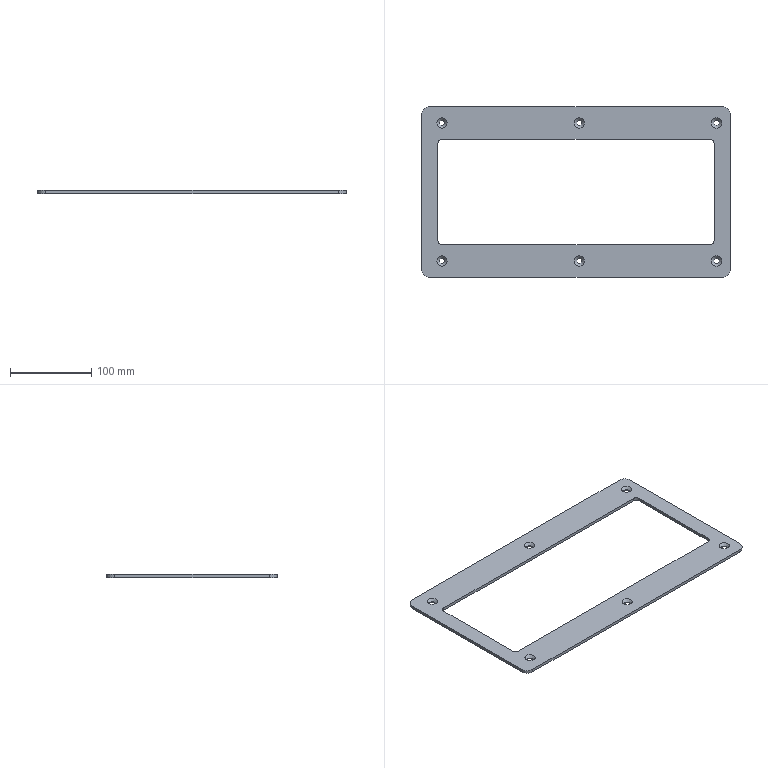Part | NX | 1 solid | 30 faces | box 380 x 210 x 3.7 mm | volume 129993 mm3 | cylinder 14 | plane 10 | cone 6 | commonest cylinder face diameters 6.6 x6 10 x4 20 x4
STEP:
#1=CARTESIAN_POINT('',(-168.3,85.,-3.7));
#2=VERTEX_POINT('',#1);
#3=CARTESIAN_POINT('',(-165.,85.,-3.7));
#4=DIRECTION('',(0.,0.,-1.));
#5=DIRECTION('',(-1.,0.,0.));
#6=AXIS2_PLACEMENT_3D('',#3,#4,#5);
#7=CIRCLE('',#6,3.3);
#8=EDGE_CURVE('',#2,#2,#7,.T.);
#9=ORIENTED_EDGE('',*,*,#8,.T.);
#10=EDGE_LOOP('',(#9));
#11=FACE_BOUND('',#10,.T.);
#12=CARTESIAN_POINT('',(-168.3,85.,-3.));
#13=VERTEX_POINT('',#12);
#14=CARTESIAN_POINT('',(-165.,85.,-3.));
#15=DIRECTION('',(0.,0.,1.));
#16=DIRECTION('',(-1.,0.,0.));
#17=AXIS2_PLACEMENT_3D('',#14,#15,#16);
#18=CIRCLE('',#17,3.3);
#19=EDGE_CURVE('',#13,#13,#18,.T.);
#20=ORIENTED_EDGE('',*,*,#19,.T.);
#21=EDGE_LOOP('',(#20));
#22=FACE_BOUND('',#21,.T.);
#23=CARTESIAN_POINT('',(-165.,85.,-0.000000002));
#24=DIRECTION('',(0.,0.,-1.));
#25=DIRECTION('',(1.,0.,0.));
#26=AXIS2_PLACEMENT_3D('',#23,#24,#25);
#27=CYLINDRICAL_SURFACE('',#26,3.3);
#28=ADVANCED_FACE('',(#11,#22),#27,.F.);
#29=CARTESIAN_POINT('',(-171.3,85.,-0.000000002));
#30=VERTEX_POINT('',#29);
#31=CARTESIAN_POINT('',(-165.,85.,-0.000000002));
#32=DIRECTION('',(0.,0.,-1.));
#33=DIRECTION('',(-1.,0.,0.));
#34=AXIS2_PLACEMENT_3D('',#31,#32,#33);
#35=CIRCLE('',#34,6.3);
#36=EDGE_CURVE('',#30,#30,#35,.T.);
#37=ORIENTED_EDGE('',*,*,#36,.F.);
#38=EDGE_LOOP('',(#37));
#39=FACE_BOUND('',#38,.T.);
#40=ORIENTED_EDGE('',*,*,#19,.F.);
#41=EDGE_LOOP('',(#40));
#42=FACE_BOUND('',#41,.T.);
#43=CARTESIAN_POINT('',(-165.,85.,-3.));
#44=DIRECTION('',(0.,0.,1.));
#45=DIRECTION('',(1.,0.,0.));
#46=AXIS2_PLACEMENT_3D('',#43,#44,#45);
#47=CONICAL_SURFACE('',#46,3.3,0.7854);
#48=ADVANCED_FACE('',(#39,#42),#47,.F.);
#49=CARTESIAN_POINT('',(0.7,85.,-3.7));
#50=VERTEX_POINT('',#49);
#51=CARTESIAN_POINT('',(4.,85.,-3.7));
#52=DIRECTION('',(0.,0.,-1.));
#53=DIRECTION('',(-1.,0.,0.));
#54=AXIS2_PLACEMENT_3D('',#51,#52,#53);
#55=CIRCLE('',#54,3.3);
#56=EDGE_CURVE('',#50,#50,#55,.T.);
#57=ORIENTED_EDGE('',*,*,#56,.T.);
#58=EDGE_LOOP('',(#57));
#59=FACE_BOUND('',#58,.T.);
#60=CARTESIAN_POINT('',(0.7,85.,-3.));
#61=VERTEX_POINT('',#60);
#62=CARTESIAN_POINT('',(4.,85.,-3.));
#63=DIRECTION('',(0.,0.,1.));
#64=DIRECTION('',(-1.,0.,0.));
#65=AXIS2_PLACEMENT_3D('',#62,#63,#64);
#66=CIRCLE('',#65,3.3);
#67=EDGE_CURVE('',#61,#61,#66,.T.);
#68=ORIENTED_EDGE('',*,*,#67,.T.);
#69=EDGE_LOOP('',(#68));
#70=FACE_BOUND('',#69,.T.);
#71=CARTESIAN_POINT('',(4.,85.,0.));
#72=DIRECTION('',(0.,0.,-1.));
#73=DIRECTION('',(1.,0.,0.));
#74=AXIS2_PLACEMENT_3D('',#71,#72,#73);
#75=CYLINDRICAL_SURFACE('',#74,3.3);
#76=ADVANCED_FACE('',(#59,#70),#75,.F.);
#77=CARTESIAN_POINT('',(-2.3,85.,0.));
#78=VERTEX_POINT('',#77);
#79=CARTESIAN_POINT('',(4.,85.,0.));
#80=DIRECTION('',(0.,0.,-1.));
#81=DIRECTION('',(-1.,0.,0.));
#82=AXIS2_PLACEMENT_3D('',#79,#80,#81);
#83=CIRCLE('',#82,6.3);
#84=EDGE_CURVE('',#78,#78,#83,.T.);
#85=ORIENTED_EDGE('',*,*,#84,.F.);
#86=EDGE_LOOP('',(#85));
#87=FACE_BOUND('',#86,.T.);
#88=ORIENTED_EDGE('',*,*,#67,.F.);
#89=EDGE_LOOP('',(#88));
#90=FACE_BOUND('',#89,.T.);
#91=CARTESIAN_POINT('',(4.,85.,-3.));
#92=DIRECTION('',(0.,0.,1.));
#93=DIRECTION('',(1.,0.,0.));
#94=AXIS2_PLACEMENT_3D('',#91,#92,#93);
#95=CONICAL_SURFACE('',#94,3.3,0.7854);
#96=ADVANCED_FACE('',(#87,#90),#95,.F.);
#97=CARTESIAN_POINT('',(169.7,85.,-3.7));
#98=VERTEX_POINT('',#97);
#99=CARTESIAN_POINT('',(173.,85.,-3.7));
#100=DIRECTION('',(0.,0.,-1.));
#101=DIRECTION('',(-1.,0.,0.));
#102=AXIS2_PLACEMENT_3D('',#99,#100,#101);
#103=CIRCLE('',#102,3.3);
#104=EDGE_CURVE('',#98,#98,#103,.T.);
#105=ORIENTED_EDGE('',*,*,#104,.T.);
#106=EDGE_LOOP('',(#105));
#107=FACE_BOUND('',#106,.T.);
#108=CARTESIAN_POINT('',(169.7,85.,-3.));
#109=VERTEX_POINT('',#108);
#110=CARTESIAN_POINT('',(173.,85.,-3.));
#111=DIRECTION('',(0.,0.,1.));
#112=DIRECTION('',(-1.,0.,0.));
#113=AXIS2_PLACEMENT_3D('',#110,#111,#112);
#114=CIRCLE('',#113,3.3);
#115=EDGE_CURVE('',#109,#109,#114,.T.);
#116=ORIENTED_EDGE('',*,*,#115,.T.);
#117=EDGE_LOOP('',(#116));
#118=FACE_BOUND('',#117,.T.);
#119=CARTESIAN_POINT('',(173.,85.,0.000000002));
#120=DIRECTION('',(0.,0.,-1.));
#121=DIRECTION('',(1.,0.,0.));
#122=AXIS2_PLACEMENT_3D('',#119,#120,#121);
#123=CYLINDRICAL_SURFACE('',#122,3.3);
#124=ADVANCED_FACE('',(#107,#118),#123,.F.);
#125=CARTESIAN_POINT('',(166.7,85.,0.000000002));
#126=VERTEX_POINT('',#125);
#127=CARTESIAN_POINT('',(173.,85.,0.000000002));
#128=DIRECTION('',(0.,0.,-1.));
#129=DIRECTION('',(-1.,0.,0.));
#130=AXIS2_PLACEMENT_3D('',#127,#128,#129);
#131=CIRCLE('',#130,6.3);
#132=EDGE_CURVE('',#126,#126,#131,.T.);
#133=ORIENTED_EDGE('',*,*,#132,.F.);
#134=EDGE_LOOP('',(#133));
#135=FACE_BOUND('',#134,.T.);
#136=ORIENTED_EDGE('',*,*,#115,.F.);
#137=EDGE_LOOP('',(#136));
#138=FACE_BOUND('',#137,.T.);
#139=CARTESIAN_POINT('',(173.,85.,-3.));
#140=DIRECTION('',(0.,0.,1.));
#141=DIRECTION('',(1.,0.,0.));
#142=AXIS2_PLACEMENT_3D('',#139,#140,#141);
#143=CONICAL_SURFACE('',#142,3.3,0.7854);
#144=ADVANCED_FACE('',(#135,#138),#143,.F.);
#145=CARTESIAN_POINT('',(-168.3,-85.,-3.7));
#146=VERTEX_POINT('',#145);
#147=CARTESIAN_POINT('',(-165.,-85.,-3.7));
#148=DIRECTION('',(0.,0.,-1.));
#149=DIRECTION('',(-1.,0.,0.));
#150=AXIS2_PLACEMENT_3D('',#147,#148,#149);
#151=CIRCLE('',#150,3.3);
#152=EDGE_CURVE('',#146,#146,#151,.T.);
#153=ORIENTED_EDGE('',*,*,#152,.T.);
#154=EDGE_LOOP('',(#153));
#155=FACE_BOUND('',#154,.T.);
#156=CARTESIAN_POINT('',(-168.3,-85.,-3.));
#157=VERTEX_POINT('',#156);
#158=CARTESIAN_POINT('',(-165.,-85.,-3.));
#159=DIRECTION('',(0.,0.,1.));
#160=DIRECTION('',(-1.,0.,0.));
#161=AXIS2_PLACEMENT_3D('',#158,#159,#160);
#162=CIRCLE('',#161,3.3);
#163=EDGE_CURVE('',#157,#157,#162,.T.);
#164=ORIENTED_EDGE('',*,*,#163,.T.);
#165=EDGE_LOOP('',(#164));
#166=FACE_BOUND('',#165,.T.);
#167=CARTESIAN_POINT('',(-165.,-85.,-0.000000004));
#168=DIRECTION('',(0.,0.,-1.));
#169=DIRECTION('',(1.,0.,0.));
#170=AXIS2_PLACEMENT_3D('',#167,#168,#169);
#171=CYLINDRICAL_SURFACE('',#170,3.3);
#172=ADVANCED_FACE('',(#155,#166),#171,.F.);
#173=CARTESIAN_POINT('',(-171.3,-85.,-0.000000004));
#174=VERTEX_POINT('',#173);
#175=CARTESIAN_POINT('',(-165.,-85.,-0.000000004));
#176=DIRECTION('',(0.,0.,-1.));
#177=DIRECTION('',(-1.,0.,0.));
#178=AXIS2_PLACEMENT_3D('',#175,#176,#177);
#179=CIRCLE('',#178,6.3);
#180=EDGE_CURVE('',#174,#174,#179,.T.);
#181=ORIENTED_EDGE('',*,*,#180,.F.);
#182=EDGE_LOOP('',(#181));
#183=FACE_BOUND('',#182,.T.);
#184=ORIENTED_EDGE('',*,*,#163,.F.);
#185=EDGE_LOOP('',(#184));
#186=FACE_BOUND('',#185,.T.);
#187=CARTESIAN_POINT('',(-165.,-85.,-3.));
#188=DIRECTION('',(0.,0.,1.));
#189=DIRECTION('',(1.,0.,0.));
#190=AXIS2_PLACEMENT_3D('',#187,#188,#189);
#191=CONICAL_SURFACE('',#190,3.3,0.7854);
#192=ADVANCED_FACE('',(#183,#186),#191,.F.);
#193=CARTESIAN_POINT('',(0.7,-85.,-3.7));
#194=VERTEX_POINT('',#193);
#195=CARTESIAN_POINT('',(4.,-85.,-3.7));
#196=DIRECTION('',(0.,0.,-1.));
#197=DIRECTION('',(-1.,0.,0.));
#198=AXIS2_PLACEMENT_3D('',#195,#196,#197);
#199=CIRCLE('',#198,3.3);
#200=EDGE_CURVE('',#194,#194,#199,.T.);
#201=ORIENTED_EDGE('',*,*,#200,.T.);
#202=EDGE_LOOP('',(#201));
#203=FACE_BOUND('',#202,.T.);
#204=CARTESIAN_POINT('',(0.7,-85.,-3.));
#205=VERTEX_POINT('',#204);
#206=CARTESIAN_POINT('',(4.,-85.,-3.));
#207=DIRECTION('',(0.,0.,1.));
#208=DIRECTION('',(-1.,0.,0.));
#209=AXIS2_PLACEMENT_3D('',#206,#207,#208);
#210=CIRCLE('',#209,3.3);
#211=EDGE_CURVE('',#205,#205,#210,.T.);
#212=ORIENTED_EDGE('',*,*,#211,.T.);
#213=EDGE_LOOP('',(#212));
#214=FACE_BOUND('',#213,.T.);
#215=CARTESIAN_POINT('',(4.,-85.,-0.000000002));
#216=DIRECTION('',(0.,0.,-1.));
#217=DIRECTION('',(1.,0.,0.));
#218=AXIS2_PLACEMENT_3D('',#215,#216,#217);
#219=CYLINDRICAL_SURFACE('',#218,3.3);
#220=ADVANCED_FACE('',(#203,#214),#219,.F.);
#221=CARTESIAN_POINT('',(-2.3,-85.,-0.000000002));
#222=VERTEX_POINT('',#221);
#223=CARTESIAN_POINT('',(4.,-85.,-0.000000002));
#224=DIRECTION('',(0.,0.,-1.));
#225=DIRECTION('',(-1.,0.,0.));
#226=AXIS2_PLACEMENT_3D('',#223,#224,#225);
#227=CIRCLE('',#226,6.3);
#228=EDGE_CURVE('',#222,#222,#227,.T.);
#229=ORIENTED_EDGE('',*,*,#228,.F.);
#230=EDGE_LOOP('',(#229));
#231=FACE_BOUND('',#230,.T.);
#232=ORIENTED_EDGE('',*,*,#211,.F.);
#233=EDGE_LOOP('',(#232));
#234=FACE_BOUND('',#233,.T.);
#235=CARTESIAN_POINT('',(4.,-85.,-3.));
#236=DIRECTION('',(0.,0.,1.));
#237=DIRECTION('',(1.,0.,0.));
#238=AXIS2_PLACEMENT_3D('',#235,#236,#237);
#239=CONICAL_SURFACE('',#238,3.3,0.7854);
#240=ADVANCED_FACE('',(#231,#234),#239,.F.);
#241=ORIENTED_EDGE('',*,*,#36,.T.);
#242=EDGE_LOOP('',(#241));
#243=FACE_BOUND('',#242,.T.);
#244=ORIENTED_EDGE('',*,*,#84,.T.);
#245=EDGE_LOOP('',(#244));
#246=FACE_BOUND('',#245,.T.);
#247=ORIENTED_EDGE('',*,*,#132,.T.);
#248=EDGE_LOOP('',(#247));
#249=FACE_BOUND('',#248,.T.);
#250=ORIENTED_EDGE('',*,*,#180,.T.);
#251=EDGE_LOOP('',(#250));
#252=FACE_BOUND('',#251,.T.);
#253=CARTESIAN_POINT('',(165.,65.,-0.000000005));
#254=VERTEX_POINT('',#253);
#255=CARTESIAN_POINT('',(-165.,65.,-0.000000004));
#256=VERTEX_POINT('',#255);
#257=CARTESIAN_POINT('',(0.000000002,65.,0.000000003));
#258=DIRECTION('',(-1.,0.,0.));
#259=VECTOR('',#258,1000.);
#260=LINE('',#257,#259);
#261=EDGE_CURVE('',#254,#256,#260,.T.);
#262=ORIENTED_EDGE('',*,*,#261,.F.);
#263=CARTESIAN_POINT('',(170.,60.,-0.000000002));
#264=VERTEX_POINT('',#263);
#265=CARTESIAN_POINT('',(165.,60.,-0.000000005));
#266=DIRECTION('',(0.,0.,1.));
#267=DIRECTION('',(-1.,0.,0.));
#268=AXIS2_PLACEMENT_3D('',#265,#266,#267);
#269=CIRCLE('',#268,5.);
#270=EDGE_CURVE('',#264,#254,#269,.T.);
#271=ORIENTED_EDGE('',*,*,#270,.F.);
#272=CARTESIAN_POINT('',(170.,-60.,-0.000000001));
#273=VERTEX_POINT('',#272);
#274=CARTESIAN_POINT('',(170.,-0.000000005,-0.000000006));
#275=DIRECTION('',(0.,1.,0.));
#276=VECTOR('',#275,1000.);
#277=LINE('',#274,#276);
#278=EDGE_CURVE('',#273,#264,#277,.T.);
#279=ORIENTED_EDGE('',*,*,#278,.F.);
#280=CARTESIAN_POINT('',(165.,-65.,-0.000000004));
#281=VERTEX_POINT('',#280);
#282=CARTESIAN_POINT('',(165.,-60.,-0.000000004));
#283=DIRECTION('',(0.,0.,1.));
#284=DIRECTION('',(-1.,0.,0.));
#285=AXIS2_PLACEMENT_3D('',#282,#283,#284);
#286=CIRCLE('',#285,5.);
#287=EDGE_CURVE('',#281,#273,#286,.T.);
#288=ORIENTED_EDGE('',*,*,#287,.F.);
#289=CARTESIAN_POINT('',(-165.,-65.,-0.000000003));
#290=VERTEX_POINT('',#289);
#291=CARTESIAN_POINT('',(-0.000000002,-65.,0.000000003));
#292=DIRECTION('',(1.,0.,0.));
#293=VECTOR('',#292,1000.);
#294=LINE('',#291,#293);
#295=EDGE_CURVE('',#290,#281,#294,.T.);
#296=ORIENTED_EDGE('',*,*,#295,.F.);
#297=CARTESIAN_POINT('',(-170.,-60.,-0.000000006));
#298=VERTEX_POINT('',#297);
#299=CARTESIAN_POINT('',(-165.,-60.,-0.000000003));
#300=DIRECTION('',(0.,0.,1.));
#301=DIRECTION('',(-1.,0.,0.));
#302=AXIS2_PLACEMENT_3D('',#299,#300,#301);
#303=CIRCLE('',#302,5.);
#304=EDGE_CURVE('',#298,#290,#303,.T.);
#305=ORIENTED_EDGE('',*,*,#304,.F.);
#306=CARTESIAN_POINT('',(-170.,60.,0.000000002));
#307=VERTEX_POINT('',#306);
#308=CARTESIAN_POINT('',(-170.,0.000000005,-0.000000002));
#309=DIRECTION('',(0.,-1.,0.));
#310=VECTOR('',#309,1000.);
#311=LINE('',#308,#310);
#312=EDGE_CURVE('',#307,#298,#311,.T.);
#313=ORIENTED_EDGE('',*,*,#312,.F.);
#314=CARTESIAN_POINT('',(-165.,60.,-0.000000004));
#315=DIRECTION('',(0.,0.,1.));
#316=DIRECTION('',(-1.,0.,0.));
#317=AXIS2_PLACEMENT_3D('',#314,#315,#316);
#318=CIRCLE('',#317,5.);
#319=EDGE_CURVE('',#256,#307,#318,.T.);
#320=ORIENTED_EDGE('',*,*,#319,.F.);
#321=EDGE_LOOP('',(#262,#271,#279,#288,#296,#305,#313,#320));
#322=FACE_BOUND('',#321,.T.);
#323=CARTESIAN_POINT('',(166.7,-85.,0.));
#324=VERTEX_POINT('',#323);
#325=CARTESIAN_POINT('',(173.,-85.,0.));
#326=DIRECTION('',(0.,0.,1.));
#327=DIRECTION('',(-1.,0.,0.));
#328=AXIS2_PLACEMENT_3D('',#325,#326,#327);
#329=CIRCLE('',#328,6.3);
#330=EDGE_CURVE('',#324,#324,#329,.T.);
#331=ORIENTED_EDGE('',*,*,#330,.F.);
#332=EDGE_LOOP('',(#331));
#333=FACE_BOUND('',#332,.T.);
#334=ORIENTED_EDGE('',*,*,#228,.T.);
#335=EDGE_LOOP('',(#334));
#336=FACE_BOUND('',#335,.T.);
#337=CARTESIAN_POINT('',(-190.,-95.,-0.000000005));
#338=VERTEX_POINT('',#337);
#339=CARTESIAN_POINT('',(-180.,-105.,0.));
#340=VERTEX_POINT('',#339);
#341=CARTESIAN_POINT('',(-180.,-95.,0.));
#342=DIRECTION('',(0.,0.,1.));
#343=DIRECTION('',(-1.,0.,0.));
#344=AXIS2_PLACEMENT_3D('',#341,#342,#343);
#345=CIRCLE('',#344,10.);
#346=EDGE_CURVE('',#338,#340,#345,.T.);
#347=ORIENTED_EDGE('',*,*,#346,.T.);
#348=CARTESIAN_POINT('',(180.,-105.,0.000000001));
#349=VERTEX_POINT('',#348);
#350=CARTESIAN_POINT('',(-0.000000002,-105.,0.));
#351=DIRECTION('',(1.,0.,0.));
#352=VECTOR('',#351,1000.);
#353=LINE('',#350,#352);
#354=EDGE_CURVE('',#340,#349,#353,.T.);
#355=ORIENTED_EDGE('',*,*,#354,.T.);
#356=CARTESIAN_POINT('',(190.,-95.,-0.000000006));
#357=VERTEX_POINT('',#356);
#358=CARTESIAN_POINT('',(180.,-95.,0.000000002));
#359=DIRECTION('',(0.,0.,1.));
#360=DIRECTION('',(-1.,0.,0.));
#361=AXIS2_PLACEMENT_3D('',#358,#359,#360);
#362=CIRCLE('',#361,10.);
#363=EDGE_CURVE('',#349,#357,#362,.T.);
#364=ORIENTED_EDGE('',*,*,#363,.T.);
#365=CARTESIAN_POINT('',(190.,95.,-0.000000003));
#366=VERTEX_POINT('',#365);
#367=CARTESIAN_POINT('',(190.,-0.000000006,0.));
#368=DIRECTION('',(0.,1.,0.));
#369=VECTOR('',#368,1000.);
#370=LINE('',#367,#369);
#371=EDGE_CURVE('',#357,#366,#370,.T.);
#372=ORIENTED_EDGE('',*,*,#371,.T.);
#373=CARTESIAN_POINT('',(180.,105.,-0.000000003));
#374=VERTEX_POINT('',#373);
#375=CARTESIAN_POINT('',(180.,95.,-0.000000004));
#376=DIRECTION('',(0.,0.,1.));
#377=DIRECTION('',(-1.,0.,0.));
#378=AXIS2_PLACEMENT_3D('',#375,#376,#377);
#379=CIRCLE('',#378,10.);
#380=EDGE_CURVE('',#366,#374,#379,.T.);
#381=ORIENTED_EDGE('',*,*,#380,.T.);
#382=CARTESIAN_POINT('',(-180.,105.,-0.000000005));
#383=VERTEX_POINT('',#382);
#384=CARTESIAN_POINT('',(0.000000006,105.,-0.000000004));
#385=DIRECTION('',(-1.,0.,0.));
#386=VECTOR('',#385,1000.);
#387=LINE('',#384,#386);
#388=EDGE_CURVE('',#374,#383,#387,.T.);
#389=ORIENTED_EDGE('',*,*,#388,.T.);
#390=CARTESIAN_POINT('',(-190.,95.,-0.000000001));
#391=VERTEX_POINT('',#390);
#392=CARTESIAN_POINT('',(-180.,95.,-0.000000005));
#393=DIRECTION('',(0.,0.,1.));
#394=DIRECTION('',(-1.,0.,0.));
#395=AXIS2_PLACEMENT_3D('',#392,#393,#394);
#396=CIRCLE('',#395,10.);
#397=EDGE_CURVE('',#383,#391,#396,.T.);
#398=ORIENTED_EDGE('',*,*,#397,.T.);
#399=CARTESIAN_POINT('',(-190.,0.000000006,-0.000000008));
#400=DIRECTION('',(0.,-1.,0.));
#401=VECTOR('',#400,1000.);
#402=LINE('',#399,#401);
#403=EDGE_CURVE('',#391,#338,#402,.T.);
#404=ORIENTED_EDGE('',*,*,#403,.T.);
#405=EDGE_LOOP('',(#347,#355,#364,#372,#381,#389,#398,#404));
#406=FACE_BOUND('',#405,.T.);
#407=CARTESIAN_POINT('',(-3327.101,5.2,0.));
#408=DIRECTION('',(0.,0.,-1.));
#409=DIRECTION('',(1.,0.,0.));
#410=AXIS2_PLACEMENT_3D('',#407,#408,#409);
#411=PLANE('',#410);
#412=ADVANCED_FACE('',(#243,#246,#249,#252,#322,#333,#336,#406),#411,.F.);
#413=CARTESIAN_POINT('',(-170.,60.,-3.7));
#414=VERTEX_POINT('',#413);
#415=CARTESIAN_POINT('',(-170.,60.,-1.85));
#416=DIRECTION('',(0.,0.,1.));
#417=VECTOR('',#416,1000.);
#418=LINE('',#415,#417);
#419=EDGE_CURVE('',#414,#307,#418,.T.);
#420=ORIENTED_EDGE('',*,*,#419,.T.);
#421=ORIENTED_EDGE('',*,*,#312,.T.);
#422=CARTESIAN_POINT('',(-170.,-60.,-3.7));
#423=VERTEX_POINT('',#422);
#424=CARTESIAN_POINT('',(-170.,-60.,-1.85));
#425=DIRECTION('',(0.,0.,1.));
#426=VECTOR('',#425,1000.);
#427=LINE('',#424,#426);
#428=EDGE_CURVE('',#423,#298,#427,.T.);
#429=ORIENTED_EDGE('',*,*,#428,.F.);
#430=CARTESIAN_POINT('',(-170.,0.000000005,-3.7));
#431=DIRECTION('',(0.,-1.,0.));
#432=VECTOR('',#431,1000.);
#433=LINE('',#430,#432);
#434=EDGE_CURVE('',#414,#423,#433,.T.);
#435=ORIENTED_EDGE('',*,*,#434,.F.);
#436=EDGE_LOOP('',(#420,#421,#429,#435));
#437=FACE_BOUND('',#436,.T.);
#438=CARTESIAN_POINT('',(-170.,65.,-3.7));
#439=DIRECTION('',(-1.,0.,0.));
#440=DIRECTION('',(0.,-1.,0.));
#441=AXIS2_PLACEMENT_3D('',#438,#439,#440);
#442=PLANE('',#441);
#443=ADVANCED_FACE('',(#437),#442,.F.);
#444=CARTESIAN_POINT('',(-165.,-65.,-3.7));
#445=VERTEX_POINT('',#444);
#446=CARTESIAN_POINT('',(-165.,-65.,-1.85));
#447=DIRECTION('',(0.,0.,1.));
#448=VECTOR('',#447,1000.);
#449=LINE('',#446,#448);
#450=EDGE_CURVE('',#445,#290,#449,.T.);
#451=ORIENTED_EDGE('',*,*,#450,.T.);
#452=ORIENTED_EDGE('',*,*,#295,.T.);
#453=CARTESIAN_POINT('',(165.,-65.,-3.7));
#454=VERTEX_POINT('',#453);
#455=CARTESIAN_POINT('',(165.,-65.,-1.85));
#456=DIRECTION('',(0.,0.,1.));
#457=VECTOR('',#456,1000.);
#458=LINE('',#455,#457);
#459=EDGE_CURVE('',#454,#281,#458,.T.);
#460=ORIENTED_EDGE('',*,*,#459,.F.);
#461=CARTESIAN_POINT('',(-0.00000001,-65.,-3.7));
#462=DIRECTION('',(1.,0.,0.));
#463=VECTOR('',#462,1000.);
#464=LINE('',#461,#463);
#465=EDGE_CURVE('',#445,#454,#464,.T.);
#466=ORIENTED_EDGE('',*,*,#465,.F.);
#467=EDGE_LOOP('',(#451,#452,#460,#466));
#468=FACE_BOUND('',#467,.T.);
#469=CARTESIAN_POINT('',(-170.,-65.,-3.7));
#470=DIRECTION('',(0.,-1.,0.));
#471=DIRECTION('',(1.,0.,0.));
#472=AXIS2_PLACEMENT_3D('',#469,#470,#471);
#473=PLANE('',#472);
#474=ADVANCED_FACE('',(#468),#473,.F.);
#475=CARTESIAN_POINT('',(170.,-60.,-3.7));
#476=VERTEX_POINT('',#475);
#477=CARTESIAN_POINT('',(170.,-60.,-1.85));
#478=DIRECTION('',(0.,0.,1.));
#479=VECTOR('',#478,1000.);
#480=LINE('',#477,#479);
#481=EDGE_CURVE('',#476,#273,#480,.T.);
#482=ORIENTED_EDGE('',*,*,#481,.T.);
#483=ORIENTED_EDGE('',*,*,#278,.T.);
#484=CARTESIAN_POINT('',(170.,60.,-3.7));
#485=VERTEX_POINT('',#484);
#486=CARTESIAN_POINT('',(170.,60.,-1.85));
#487=DIRECTION('',(0.,0.,1.));
#488=VECTOR('',#487,1000.);
#489=LINE('',#486,#488);
#490=EDGE_CURVE('',#485,#264,#489,.T.);
#491=ORIENTED_EDGE('',*,*,#490,.F.);
#492=CARTESIAN_POINT('',(170.,-0.000000005,-3.7));
#493=DIRECTION('',(0.,1.,0.));
#494=VECTOR('',#493,1000.);
#495=LINE('',#492,#494);
#496=EDGE_CURVE('',#476,#485,#495,.T.);
#497=ORIENTED_EDGE('',*,*,#496,.F.);
#498=EDGE_LOOP('',(#482,#483,#491,#497));
#499=FACE_BOUND('',#498,.T.);
#500=CARTESIAN_POINT('',(170.,-65.,-3.7));
#501=DIRECTION('',(1.,0.,0.));
#502=DIRECTION('',(0.,1.,0.));
#503=AXIS2_PLACEMENT_3D('',#500,#501,#502);
#504=PLANE('',#503);
#505=ADVANCED_FACE('',(#499),#504,.F.);
#506=CARTESIAN_POINT('',(-165.,65.,-3.7));
#507=VERTEX_POINT('',#506);
#508=CARTESIAN_POINT('',(-165.,65.,-1.85));
#509=DIRECTION('',(0.,0.,1.));
#510=VECTOR('',#509,1000.);
#511=LINE('',#508,#510);
#512=EDGE_CURVE('',#507,#256,#511,.T.);
#513=ORIENTED_EDGE('',*,*,#512,.F.);
#514=CARTESIAN_POINT('',(165.,65.,-3.7));
#515=VERTEX_POINT('',#514);
#516=CARTESIAN_POINT('',(-0.000000006,65.,-3.7));
#517=DIRECTION('',(-1.,0.,0.));
#518=VECTOR('',#517,1000.);
#519=LINE('',#516,#518);
#520=EDGE_CURVE('',#515,#507,#519,.T.);
#521=ORIENTED_EDGE('',*,*,#520,.F.);
#522=CARTESIAN_POINT('',(165.,65.,-1.85));
#523=DIRECTION('',(0.,0.,1.));
#524=VECTOR('',#523,1000.);
#525=LINE('',#522,#524);
#526=EDGE_CURVE('',#515,#254,#525,.T.);
#527=ORIENTED_EDGE('',*,*,#526,.T.);
#528=ORIENTED_EDGE('',*,*,#261,.T.);
#529=EDGE_LOOP('',(#513,#521,#527,#528));
#530=FACE_BOUND('',#529,.T.);
#531=CARTESIAN_POINT('',(170.,65.,-3.7));
#532=DIRECTION('',(0.,1.,0.));
#533=DIRECTION('',(-1.,0.,0.));
#534=AXIS2_PLACEMENT_3D('',#531,#532,#533);
#535=PLANE('',#534);
#536=ADVANCED_FACE('',(#530),#535,.F.);
#537=ORIENTED_EDGE('',*,*,#490,.T.);
#538=ORIENTED_EDGE('',*,*,#270,.T.);
#539=ORIENTED_EDGE('',*,*,#526,.F.);
#540=CARTESIAN_POINT('',(165.,60.,-3.7));
#541=DIRECTION('',(0.,0.,-1.));
#542=DIRECTION('',(-1.,0.,0.));
#543=AXIS2_PLACEMENT_3D('',#540,#541,#542);
#544=CIRCLE('',#543,5.);
#545=EDGE_CURVE('',#515,#485,#544,.T.);
#546=ORIENTED_EDGE('',*,*,#545,.T.);
#547=EDGE_LOOP('',(#537,#538,#539,#546));
#548=FACE_BOUND('',#547,.T.);
#549=CARTESIAN_POINT('',(165.,60.,-1.85));
#550=DIRECTION('',(0.,0.,1.));
#551=DIRECTION('',(1.,0.,0.));
#552=AXIS2_PLACEMENT_3D('',#549,#550,#551);
#553=CYLINDRICAL_SURFACE('',#552,5.);
#554=ADVANCED_FACE('',(#548),#553,.F.);
#555=ORIENTED_EDGE('',*,*,#459,.T.);
#556=ORIENTED_EDGE('',*,*,#287,.T.);
#557=ORIENTED_EDGE('',*,*,#481,.F.);
#558=CARTESIAN_POINT('',(165.,-60.,-3.7));
#559=DIRECTION('',(0.,0.,-1.));
#560=DIRECTION('',(-1.,0.,0.));
#561=AXIS2_PLACEMENT_3D('',#558,#559,#560);
#562=CIRCLE('',#561,5.);
#563=EDGE_CURVE('',#476,#454,#562,.T.);
#564=ORIENTED_EDGE('',*,*,#563,.T.);
#565=EDGE_LOOP('',(#555,#556,#557,#564));
#566=FACE_BOUND('',#565,.T.);
#567=CARTESIAN_POINT('',(165.,-60.,-1.85));
#568=DIRECTION('',(0.,0.,1.));
#569=DIRECTION('',(0.,-1.,0.));
#570=AXIS2_PLACEMENT_3D('',#567,#568,#569);
#571=CYLINDRICAL_SURFACE('',#570,5.);
#572=ADVANCED_FACE('',(#566),#571,.F.);
#573=ORIENTED_EDGE('',*,*,#428,.T.);
#574=ORIENTED_EDGE('',*,*,#304,.T.);
#575=ORIENTED_EDGE('',*,*,#450,.F.);
#576=CARTESIAN_POINT('',(-165.,-60.,-3.7));
#577=DIRECTION('',(0.,0.,-1.));
#578=DIRECTION('',(-1.,0.,0.));
#579=AXIS2_PLACEMENT_3D('',#576,#577,#578);
#580=CIRCLE('',#579,5.);
#581=EDGE_CURVE('',#445,#423,#580,.T.);
#582=ORIENTED_EDGE('',*,*,#581,.T.);
#583=EDGE_LOOP('',(#573,#574,#575,#582));
#584=FACE_BOUND('',#583,.T.);
#585=CARTESIAN_POINT('',(-165.,-60.,-1.85));
#586=DIRECTION('',(0.,0.,1.));
#587=DIRECTION('',(-1.,0.,0.));
#588=AXIS2_PLACEMENT_3D('',#585,#586,#587);
#589=CYLINDRICAL_SURFACE('',#588,5.);
#590=ADVANCED_FACE('',(#584),#589,.F.);
#591=ORIENTED_EDGE('',*,*,#512,.T.);
#592=ORIENTED_EDGE('',*,*,#319,.T.);
#593=ORIENTED_EDGE('',*,*,#419,.F.);
#594=CARTESIAN_POINT('',(-165.,60.,-3.7));
#595=DIRECTION('',(0.,0.,-1.));
#596=DIRECTION('',(-1.,0.,0.));
#597=AXIS2_PLACEMENT_3D('',#594,#595,#596);
#598=CIRCLE('',#597,5.);
#599=EDGE_CURVE('',#414,#507,#598,.T.);
#600=ORIENTED_EDGE('',*,*,#599,.T.);
#601=EDGE_LOOP('',(#591,#592,#593,#600));
#602=FACE_BOUND('',#601,.T.);
#603=CARTESIAN_POINT('',(-165.,60.,-1.85));
#604=DIRECTION('',(0.,0.,1.));
#605=DIRECTION('',(0.,1.,0.));
#606=AXIS2_PLACEMENT_3D('',#603,#604,#605);
#607=CYLINDRICAL_SURFACE('',#606,5.);
#608=ADVANCED_FACE('',(#602),#607,.F.);
#609=ORIENTED_EDGE('',*,*,#371,.F.);
#610=CARTESIAN_POINT('',(190.,-95.,-3.7));
#611=VERTEX_POINT('',#610);
#612=CARTESIAN_POINT('',(190.,-95.,-1.85));
#613=DIRECTION('',(0.,0.,1.));
#614=VECTOR('',#613,1000.);
#615=LINE('',#612,#614);
#616=EDGE_CURVE('',#611,#357,#615,.T.);
#617=ORIENTED_EDGE('',*,*,#616,.F.);
#618=CARTESIAN_POINT('',(190.,95.,-3.7));
#619=VERTEX_POINT('',#618);
#620=CARTESIAN_POINT('',(190.,-0.000000006,-3.7));
#621=DIRECTION('',(0.,1.,0.));
#622=VECTOR('',#621,1000.);
#623=LINE('',#620,#622);
#624=EDGE_CURVE('',#611,#619,#623,.T.);
#625=ORIENTED_EDGE('',*,*,#624,.T.);
#626=CARTESIAN_POINT('',(190.,95.,-1.85));
#627=DIRECTION('',(0.,0.,1.));
#628=VECTOR('',#627,1000.);
#629=LINE('',#626,#628);
#630=EDGE_CURVE('',#619,#366,#629,.T.);
#631=ORIENTED_EDGE('',*,*,#630,.T.);
#632=EDGE_LOOP('',(#609,#617,#625,#631));
#633=FACE_BOUND('',#632,.T.);
#634=CARTESIAN_POINT('',(190.,-105.,-3.7));
#635=DIRECTION('',(1.,0.,0.));
#636=DIRECTION('',(0.,1.,0.));
#637=AXIS2_PLACEMENT_3D('',#634,#635,#636);
#638=PLANE('',#637);
#639=ADVANCED_FACE('',(#633),#638,.T.);
#640=ORIENTED_EDGE('',*,*,#380,.F.);
#641=ORIENTED_EDGE('',*,*,#630,.F.);
#642=CARTESIAN_POINT('',(180.,105.,-3.7));
#643=VERTEX_POINT('',#642);
#644=CARTESIAN_POINT('',(180.,95.,-3.7));
#645=DIRECTION('',(0.,0.,-1.));
#646=DIRECTION('',(-1.,0.,0.));
#647=AXIS2_PLACEMENT_3D('',#644,#645,#646);
#648=CIRCLE('',#647,10.);
#649=EDGE_CURVE('',#643,#619,#648,.T.);
#650=ORIENTED_EDGE('',*,*,#649,.F.);
#651=CARTESIAN_POINT('',(180.,105.,-1.85));
#652=DIRECTION('',(0.,0.,1.));
#653=VECTOR('',#652,1000.);
#654=LINE('',#651,#653);
#655=EDGE_CURVE('',#643,#374,#654,.T.);
#656=ORIENTED_EDGE('',*,*,#655,.T.);
#657=EDGE_LOOP('',(#640,#641,#650,#656));
#658=FACE_BOUND('',#657,.T.);
#659=CARTESIAN_POINT('',(180.,95.,-1.85));
#660=DIRECTION('',(0.,0.,1.));
#661=DIRECTION('',(1.,0.,0.));
#662=AXIS2_PLACEMENT_3D('',#659,#660,#661);
#663=CYLINDRICAL_SURFACE('',#662,10.);
#664=ADVANCED_FACE('',(#658),#663,.T.);
#665=ORIENTED_EDGE('',*,*,#388,.F.);
#666=ORIENTED_EDGE('',*,*,#655,.F.);
#667=CARTESIAN_POINT('',(-180.,105.,-3.7));
#668=VERTEX_POINT('',#667);
#669=CARTESIAN_POINT('',(-0.000000001,105.,-3.7));
#670=DIRECTION('',(-1.,0.,0.));
#671=VECTOR('',#670,1000.);
#672=LINE('',#669,#671);
#673=EDGE_CURVE('',#643,#668,#672,.T.);
#674=ORIENTED_EDGE('',*,*,#673,.T.);
#675=CARTESIAN_POINT('',(-180.,105.,-1.85));
#676=DIRECTION('',(0.,0.,1.));
#677=VECTOR('',#676,1000.);
#678=LINE('',#675,#677);
#679=EDGE_CURVE('',#668,#383,#678,.T.);
#680=ORIENTED_EDGE('',*,*,#679,.T.);
#681=EDGE_LOOP('',(#665,#666,#674,#680));
#682=FACE_BOUND('',#681,.T.);
#683=CARTESIAN_POINT('',(190.,105.,-3.7));
#684=DIRECTION('',(0.,1.,0.));
#685=DIRECTION('',(-1.,0.,0.));
#686=AXIS2_PLACEMENT_3D('',#683,#684,#685);
#687=PLANE('',#686);
#688=ADVANCED_FACE('',(#682),#687,.T.);
#689=ORIENTED_EDGE('',*,*,#397,.F.);
#690=ORIENTED_EDGE('',*,*,#679,.F.);
#691=CARTESIAN_POINT('',(-190.,95.,-3.7));
#692=VERTEX_POINT('',#691);
#693=CARTESIAN_POINT('',(-180.,95.,-3.7));
#694=DIRECTION('',(0.,0.,-1.));
#695=DIRECTION('',(-1.,0.,0.));
#696=AXIS2_PLACEMENT_3D('',#693,#694,#695);
#697=CIRCLE('',#696,10.);
#698=EDGE_CURVE('',#692,#668,#697,.T.);
#699=ORIENTED_EDGE('',*,*,#698,.F.);
#700=CARTESIAN_POINT('',(-190.,95.,-1.85));
#701=DIRECTION('',(0.,0.,1.));
#702=VECTOR('',#701,1000.);
#703=LINE('',#700,#702);
#704=EDGE_CURVE('',#692,#391,#703,.T.);
#705=ORIENTED_EDGE('',*,*,#704,.T.);
#706=EDGE_LOOP('',(#689,#690,#699,#705));
#707=FACE_BOUND('',#706,.T.);
#708=CARTESIAN_POINT('',(-180.,95.,-1.85));
#709=DIRECTION('',(0.,0.,1.));
#710=DIRECTION('',(0.,1.,0.));
#711=AXIS2_PLACEMENT_3D('',#708,#709,#710);
#712=CYLINDRICAL_SURFACE('',#711,10.);
#713=ADVANCED_FACE('',(#707),#712,.T.);
#714=ORIENTED_EDGE('',*,*,#403,.F.);
#715=ORIENTED_EDGE('',*,*,#704,.F.);
#716=CARTESIAN_POINT('',(-190.,-95.,-3.7));
#717=VERTEX_POINT('',#716);
#718=CARTESIAN_POINT('',(-190.,0.000000006,-3.7));
#719=DIRECTION('',(0.,-1.,0.));
#720=VECTOR('',#719,1000.);
#721=LINE('',#718,#720);
#722=EDGE_CURVE('',#692,#717,#721,.T.);
#723=ORIENTED_EDGE('',*,*,#722,.T.);
#724=CARTESIAN_POINT('',(-190.,-95.,-1.85));
#725=DIRECTION('',(0.,0.,1.));
#726=VECTOR('',#725,1000.);
#727=LINE('',#724,#726);
#728=EDGE_CURVE('',#717,#338,#727,.T.);
#729=ORIENTED_EDGE('',*,*,#728,.T.);
#730=EDGE_LOOP('',(#714,#715,#723,#729));
#731=FACE_BOUND('',#730,.T.);
#732=CARTESIAN_POINT('',(-190.,105.,-3.7));
#733=DIRECTION('',(-1.,0.,0.));
#734=DIRECTION('',(0.,-1.,0.));
#735=AXIS2_PLACEMENT_3D('',#732,#733,#734);
#736=PLANE('',#735);
#737=ADVANCED_FACE('',(#731),#736,.T.);
#738=ORIENTED_EDGE('',*,*,#363,.F.);
#739=CARTESIAN_POINT('',(180.,-105.,-3.7));
#740=VERTEX_POINT('',#739);
#741=CARTESIAN_POINT('',(180.,-105.,-1.85));
#742=DIRECTION('',(0.,0.,1.));
#743=VECTOR('',#742,1000.);
#744=LINE('',#741,#743);
#745=EDGE_CURVE('',#740,#349,#744,.T.);
#746=ORIENTED_EDGE('',*,*,#745,.F.);
#747=CARTESIAN_POINT('',(180.,-95.,-3.7));
#748=DIRECTION('',(0.,0.,-1.));
#749=DIRECTION('',(-1.,0.,0.));
#750=AXIS2_PLACEMENT_3D('',#747,#748,#749);
#751=CIRCLE('',#750,10.);
#752=EDGE_CURVE('',#611,#740,#751,.T.);
#753=ORIENTED_EDGE('',*,*,#752,.F.);
#754=ORIENTED_EDGE('',*,*,#616,.T.);
#755=EDGE_LOOP('',(#738,#746,#753,#754));
#756=FACE_BOUND('',#755,.T.);
#757=CARTESIAN_POINT('',(180.,-95.,-1.85));
#758=DIRECTION('',(0.,0.,1.));
#759=DIRECTION('',(0.,-1.,0.));
#760=AXIS2_PLACEMENT_3D('',#757,#758,#759);
#761=CYLINDRICAL_SURFACE('',#760,10.);
#762=ADVANCED_FACE('',(#756),#761,.T.);
#763=ORIENTED_EDGE('',*,*,#346,.F.);
#764=ORIENTED_EDGE('',*,*,#728,.F.);
#765=CARTESIAN_POINT('',(-180.,-105.,-3.7));
#766=VERTEX_POINT('',#765);
#767=CARTESIAN_POINT('',(-180.,-95.,-3.7));
#768=DIRECTION('',(0.,0.,-1.));
#769=DIRECTION('',(-1.,0.,0.));
#770=AXIS2_PLACEMENT_3D('',#767,#768,#769);
#771=CIRCLE('',#770,10.);
#772=EDGE_CURVE('',#766,#717,#771,.T.);
#773=ORIENTED_EDGE('',*,*,#772,.F.);
#774=CARTESIAN_POINT('',(-180.,-105.,-1.85));
#775=DIRECTION('',(0.,0.,1.));
#776=VECTOR('',#775,1000.);
#777=LINE('',#774,#776);
#778=EDGE_CURVE('',#766,#340,#777,.T.);
#779=ORIENTED_EDGE('',*,*,#778,.T.);
#780=EDGE_LOOP('',(#763,#764,#773,#779));
#781=FACE_BOUND('',#780,.T.);
#782=CARTESIAN_POINT('',(-180.,-95.,-1.85));
#783=DIRECTION('',(0.,0.,1.));
#784=DIRECTION('',(-1.,0.,0.));
#785=AXIS2_PLACEMENT_3D('',#782,#783,#784);
#786=CYLINDRICAL_SURFACE('',#785,10.);
#787=ADVANCED_FACE('',(#781),#786,.T.);
#788=CARTESIAN_POINT('',(-0.00000001,-105.,-3.7));
#789=DIRECTION('',(1.,0.,0.));
#790=VECTOR('',#789,1000.);
#791=LINE('',#788,#790);
#792=EDGE_CURVE('',#766,#740,#791,.T.);
#793=ORIENTED_EDGE('',*,*,#792,.T.);
#794=ORIENTED_EDGE('',*,*,#745,.T.);
#795=ORIENTED_EDGE('',*,*,#354,.F.);
#796=ORIENTED_EDGE('',*,*,#778,.F.);
#797=EDGE_LOOP('',(#793,#794,#795,#796));
#798=FACE_BOUND('',#797,.T.);
#799=CARTESIAN_POINT('',(-190.,-105.,-3.7));
#800=DIRECTION('',(0.,-1.,0.));
#801=DIRECTION('',(1.,0.,0.));
#802=AXIS2_PLACEMENT_3D('',#799,#800,#801);
#803=PLANE('',#802);
#804=ADVANCED_FACE('',(#798),#803,.T.);
#805=ORIENTED_EDGE('',*,*,#8,.F.);
#806=EDGE_LOOP('',(#805));
#807=FACE_BOUND('',#806,.T.);
#808=ORIENTED_EDGE('',*,*,#56,.F.);
#809=EDGE_LOOP('',(#808));
#810=FACE_BOUND('',#809,.T.);
#811=ORIENTED_EDGE('',*,*,#104,.F.);
#812=EDGE_LOOP('',(#811));
#813=FACE_BOUND('',#812,.T.);
#814=ORIENTED_EDGE('',*,*,#152,.F.);
#815=EDGE_LOOP('',(#814));
#816=FACE_BOUND('',#815,.T.);
#817=ORIENTED_EDGE('',*,*,#599,.F.);
#818=ORIENTED_EDGE('',*,*,#434,.T.);
#819=ORIENTED_EDGE('',*,*,#581,.F.);
#820=ORIENTED_EDGE('',*,*,#465,.T.);
#821=ORIENTED_EDGE('',*,*,#563,.F.);
#822=ORIENTED_EDGE('',*,*,#496,.T.);
#823=ORIENTED_EDGE('',*,*,#545,.F.);
#824=ORIENTED_EDGE('',*,*,#520,.T.);
#825=EDGE_LOOP('',(#817,#818,#819,#820,#821,#822,#823,#824));
#826=FACE_BOUND('',#825,.T.);
#827=CARTESIAN_POINT('',(169.7,-85.,-3.7));
#828=VERTEX_POINT('',#827);
#829=CARTESIAN_POINT('',(173.,-85.,-3.7));
#830=DIRECTION('',(0.,0.,-1.));
#831=DIRECTION('',(-1.,0.,0.));
#832=AXIS2_PLACEMENT_3D('',#829,#830,#831);
#833=CIRCLE('',#832,3.3);
#834=EDGE_CURVE('',#828,#828,#833,.T.);
#835=ORIENTED_EDGE('',*,*,#834,.F.);
#836=EDGE_LOOP('',(#835));
#837=FACE_BOUND('',#836,.T.);
#838=ORIENTED_EDGE('',*,*,#200,.F.);
#839=EDGE_LOOP('',(#838));
#840=FACE_BOUND('',#839,.T.);
#841=ORIENTED_EDGE('',*,*,#722,.F.);
#842=ORIENTED_EDGE('',*,*,#698,.T.);
#843=ORIENTED_EDGE('',*,*,#673,.F.);
#844=ORIENTED_EDGE('',*,*,#649,.T.);
#845=ORIENTED_EDGE('',*,*,#624,.F.);
#846=ORIENTED_EDGE('',*,*,#752,.T.);
#847=ORIENTED_EDGE('',*,*,#792,.F.);
#848=ORIENTED_EDGE('',*,*,#772,.T.);
#849=EDGE_LOOP('',(#841,#842,#843,#844,#845,#846,#847,#848));
#850=FACE_BOUND('',#849,.T.);
#851=CARTESIAN_POINT('',(-3327.101,5.2,-3.7));
#852=DIRECTION('',(0.,0.,-1.));
#853=DIRECTION('',(1.,0.,0.));
#854=AXIS2_PLACEMENT_3D('',#851,#852,#853);
#855=PLANE('',#854);
#856=ADVANCED_FACE('',(#807,#810,#813,#816,#826,#837,#840,#850),#855,.T.);
#857=ORIENTED_EDGE('',*,*,#834,.T.);
#858=EDGE_LOOP('',(#857));
#859=FACE_BOUND('',#858,.T.);
#860=CARTESIAN_POINT('',(169.7,-85.,-3.));
#861=VERTEX_POINT('',#860);
#862=CARTESIAN_POINT('',(173.,-85.,-3.));
#863=DIRECTION('',(0.,0.,1.));
#864=DIRECTION('',(-1.,0.,0.));
#865=AXIS2_PLACEMENT_3D('',#862,#863,#864);
#866=CIRCLE('',#865,3.3);
#867=EDGE_CURVE('',#861,#861,#866,.T.);
#868=ORIENTED_EDGE('',*,*,#867,.T.);
#869=EDGE_LOOP('',(#868));
#870=FACE_BOUND('',#869,.T.);
#871=CARTESIAN_POINT('',(173.,-85.,0.));
#872=DIRECTION('',(0.,0.,-1.));
#873=DIRECTION('',(1.,0.,0.));
#874=AXIS2_PLACEMENT_3D('',#871,#872,#873);
#875=CYLINDRICAL_SURFACE('',#874,3.3);
#876=ADVANCED_FACE('',(#859,#870),#875,.F.);
#877=ORIENTED_EDGE('',*,*,#330,.T.);
#878=EDGE_LOOP('',(#877));
#879=FACE_BOUND('',#878,.T.);
#880=ORIENTED_EDGE('',*,*,#867,.F.);
#881=EDGE_LOOP('',(#880));
#882=FACE_BOUND('',#881,.T.);
#883=CARTESIAN_POINT('',(173.,-85.,-3.));
#884=DIRECTION('',(0.,0.,1.));
#885=DIRECTION('',(1.,0.,0.));
#886=AXIS2_PLACEMENT_3D('',#883,#884,#885);
#887=CONICAL_SURFACE('',#886,3.3,0.7854);
#888=ADVANCED_FACE('',(#879,#882),#887,.F.);
#889=CLOSED_SHELL('',(#28,#48,#76,#96,#124,#144,#172,#192,#220,#240,#412,#443,#474,#505,#536,#554,#572,#590,#608,#639,#664,#688,#713,#737,#762,#787,#804,#856,#876,#888));
#890=MANIFOLD_SOLID_BREP('',#889);
#891=(LENGTH_UNIT()NAMED_UNIT(*)SI_UNIT(.MILLI.,.METRE.));
#892=UNCERTAINTY_MEASURE_WITH_UNIT(LENGTH_MEASURE(0.00001),#891,'','');
#893=(NAMED_UNIT(*)PLANE_ANGLE_UNIT()SI_UNIT($,.RADIAN.));
#894=(NAMED_UNIT(*)SI_UNIT($,.STERADIAN.)SOLID_ANGLE_UNIT());
#895=(GEOMETRIC_REPRESENTATION_CONTEXT(3)GLOBAL_UNCERTAINTY_ASSIGNED_CONTEXT((#892))GLOBAL_UNIT_ASSIGNED_CONTEXT((#891,#893,#894))REPRESENTATION_CONTEXT('',''));
#896=ADVANCED_BREP_SHAPE_REPRESENTATION('',(#890),#895);